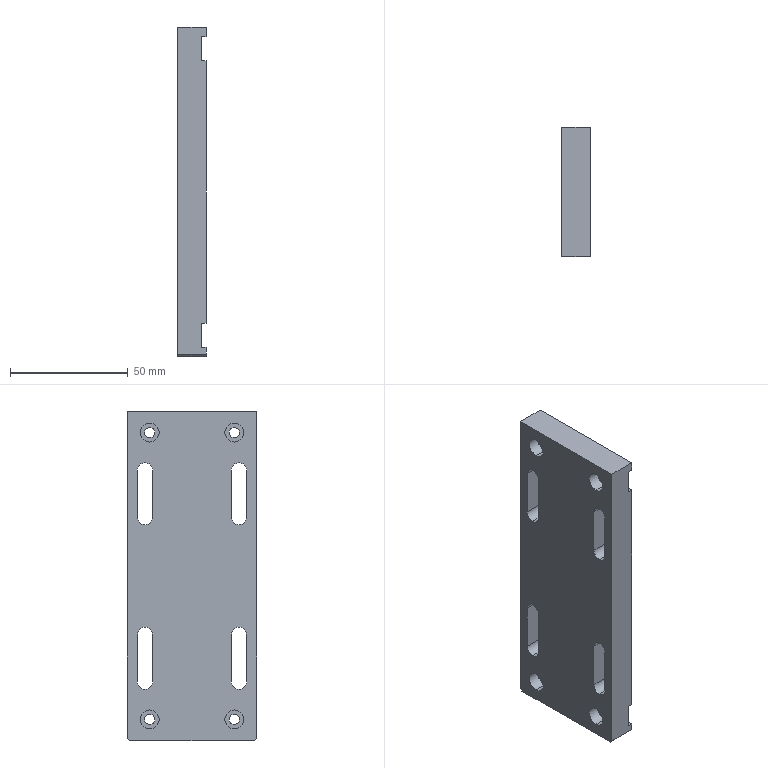Part | SolidWorks | features ICE 2, Chamfer 1, Extrusion 1, HoleWzd 1, MirrorPattern 1 | 1 solid | 56 faces | box 12 x 55 x 140 mm | volume 81002 mm3 | cylinder 28 | plane 28 | commonest cylinder face diameters 6.5 x12 4.4 x8 8 x8